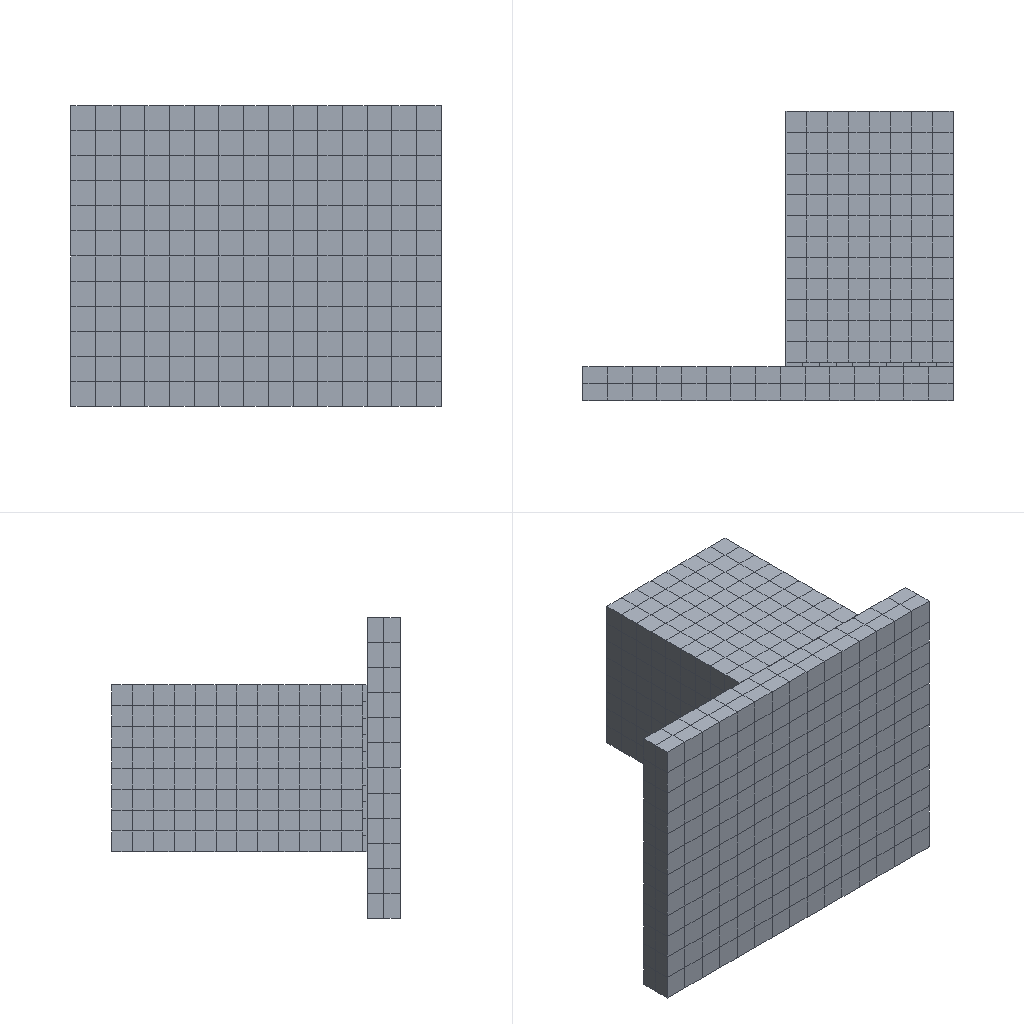Simulation study | ansys workbench
Ansys APDL input file, long lists of numbers shortened:
/batch
/config,noeldb,1     ! force off writing results to database
*get,_wallstrt,active,,time,wall
! ANSYS input file written by Workbench version 2022 R1
! File used for geometry attach:
/title,111--____ (F5)
! ****** Begin Custom Load Command Snippet ******
/COM, ACT Extensions:
/COM,     LSDYNA, 2021.1
/COM,
! ****** End   Custom Load Command Snippet ******
*DIM,_wb_ProjectScratch_dir,string,248
_wb_ProjectScratch_dir(1) = ''
*DIM,_wb_SolverFiles_dir,string,248
_wb_SolverFiles_dir(1) = ''
*DIM,_wb_userfiles_dir,string,248
_wb_userfiles_dir(1) = ''
/com,--- Data in consistent NMM units. See Solving Units in the help system for more information.
/units,MPA
/nopr
/wb,file,start              !  signify a WB generated input file
/prep7
! Turn off shape checking because checks already performed inside WB mesher.
! See help system for more information.
SHPP,OFF,,NOWARN
/nolist
etcon,set             ! allow ANSYS to choose best KEYOP's for 180x elements, resets any applicable keyopt to MAPDL defaults
/com,*********** Nodes for the whole assembly ***********
nblock,3,,7591
(1i9,3e20.9e3)
        1    -2.000000000E+00     0.000000000E+00    -2.000000000E+00
! (6900 more lines like these left out)
-1
/wb,elem,start            !  set before creation of elements
/com,*********** Elements for Body 1 "__2____1|NONE" ***********
et,1,186
keyo,1,2,1          ! set full integration on SOLID186
eblock,19,solid,,768
(19i9)
        1        1        1        1        0        0        0        0       20        0      461     3005     3858     3875     3882     3620     3859     3874     3959
! (1535 more lines like these left out)
-1
/com,*********** Elements for Body 2 "__5____1|NONE" ***********
et,2,186
keyo,2,2,1          ! set full integration on SOLID186
eblock,19,solid,,360
(19i9)
        2        2        2        2        0        0        0        0       20        0      101      804     1320     1348     1416     1111     1347     1349     1417
! (719 more lines like these left out)
-1
/com,*********** Elements for Body 3 "__3^___1|__-__1" ***********
et,3,186
keyo,3,2,1          ! set full integration on SOLID186
eblock,19,solid,,100
(19i9)
        3        3        3        3        0        0        0        0       20        0        1       81      222      223      224       82      183      182      181
! (199 more lines like these left out)
-1
/wb,elem,end               !  done creating elements
/com,*********** Send User Defined Coordinate System(s) ***********
csys,0
toffst,273.15,  ! Temperature offset from absolute zero
/com,*********** Set Reference Temperature ***********
tref,22.
/wb,mat,start              !  starting to send materials
/com,*********** Send Materials ***********
Temperature = 'TEMP' ! Temperature
MP,DENS,1,7.85e-09,	! tonne mm^-3
MP,ALPX,1,1.2e-05,	! C^-1
MP,C,1,434000000,	! mm^2 s^-2 C^-1
MP,KXX,1,60.5,	! tonne mm s^-3 C^-1
MP,RSVX,1,0.00017,	! ohm mm
MP,EX,1,200000,	! tonne s^-2 mm^-1
MP,NUXY,1,0.3,
MP,MURX,1,10000,
Temperature = 'TEMP' ! Temperature
MP,DENS,2,7.85e-09,	! tonne mm^-3
MP,ALPX,2,1.2e-05,	! C^-1
MP,C,2,434000000,	! mm^2 s^-2 C^-1
MP,KXX,2,60.5,	! tonne mm s^-3 C^-1
MP,RSVX,2,0.00017,	! ohm mm
MP,EX,2,200000,	! tonne s^-2 mm^-1
MP,NUXY,2,0.3,
MP,MURX,2,10000,
Temperature = 'TEMP' ! Temperature
MP,DENS,3,7.85e-09,	! tonne mm^-3
MP,ALPX,3,1.2e-05,	! C^-1
MP,C,3,434000000,	! mm^2 s^-2 C^-1
MP,KXX,3,60.5,	! tonne mm s^-3 C^-1
MP,RSVX,3,0.00017,	! ohm mm
MP,EX,3,200000,	! tonne s^-2 mm^-1
MP,NUXY,3,0.3,
MP,MURX,3,10000,
/wb,mat,end                !  done sending materials
!************************* Model Summary ********************
!__2____1|NONE,	结构钢,	matid,	1
!__5____1|NONE,	结构钢,	matid,	2
!__3^___1|__-__1,	结构钢,	matid,	3
!************************* End Model Summary ********************
! get the diagonal of the bounding box. Needed later for other things
*get,_xmin,node,,mnloc,x
*get,_ymin,node,,mnloc,y
*get,_zmin,node,,mnloc,z
*get,_xmax,node,,mxloc,x
*get,_ymax,node,,mxloc,y
*get,_zmax,node,,mxloc,z
_ASMDIAG=(_xmax-_xmin)*(_xmax-_xmin)+(_ymax-_ymin)*(_ymax-_ymin)+(_zmax-_zmin)*(_zmax-_zmin)
_ASMDIAG=SQRT(_ASMDIAG)
/wb,contact,start          !  starting to send contact
/com,*********** Create Contact "接触区域" ***********
/com,            Real Constant Set For Above Contact Is 5 & 4
*set,tid,5
*set,cid,4
r,tid
r,cid
et,tid,170
et,cid,174
eblock,10,,,64
(15i9)
     2449        5        5        5        0     3730     3738     3809     3729     6288     6304     6286     6285
! (63 more lines like these left out)
-1
eblock,10,,,64
(15i9)
     2513        4        4        4        0     3730     3738     3809     3729     6288     6304     6286     6285
! (63 more lines like these left out)
-1
eblock,10,,,100
(15i9)
     2577        4        5        4        0      222       81      224      223      502      503      785      784
! (99 more lines like these left out)
-1
eblock,10,,,100
(15i9)
     2677        5        4        5        0      222       81      224      223      502      503      785      784
! (99 more lines like these left out)
-1
keyo,cid,8,2               ! auto create asymmetric contact (from Program Controlled setting)
keyo,cid,10,0              ! adjust contact stiffness each NR iteration (from Program Controlled setting)
keyo,cid,12,5              ! bonded always
keyo,cid,2,0               ! augmented Lagrange
keyo,cid,4,0               ! on Gauss point (from Program Controlled setting)
keyo,cid,9,1               ! ignore initial gaps/penetration
keyo,cid,7,0               ! No Prediction
rmod,tid,3,10.      ! FKN
rmod,tid,5,0.       ! ICONT
rmod,tid,6,0.       ! PINB
rmod,tid,10,0.      ! CNOF
rmod,tid,12,0.      ! FKT
rmod,tid,36,33      ! WB DSID
rmod,cid,3,10.      ! FKN
rmod,cid,5,0.       ! ICONT
rmod,cid,6,0.       ! PINB
rmod,cid,10,0.      ! CNOF
rmod,cid,12,0.      ! FKT
rmod,cid,36,33      ! WB DSID
/com,*********** Create Contact "接触区域 2" ***********
/com,            Real Constant Set For Above Contact Is 7 & 6
*set,tid,7
*set,cid,6
r,tid
r,cid
et,tid,170
et,cid,174
eblock,10,,,56
(15i9)
     2777        7        7        7        0     1201     1202     1191     1190     2600     2580     2577     2578
! (55 more lines like these left out)
-1
eblock,10,,,56
(15i9)
     2833        6        6        6        0     1201     1202     1191     1190     2600     2580     2577     2578
! (55 more lines like these left out)
-1
eblock,10,,,100
(15i9)
     2889        6        7        6        0      181       82      183      182      506      507      723      721
! (99 more lines like these left out)
-1
eblock,10,,,100
(15i9)
     2989        7        6        7        0      181       82      183      182      506      507      723      721
! (99 more lines like these left out)
-1
keyo,cid,8,2               ! auto create asymmetric contact (from Program Controlled setting)
keyo,cid,10,0              ! adjust contact stiffness each NR iteration (from Program Controlled setting)
keyo,cid,12,5              ! bonded always
keyo,cid,2,0               ! augmented Lagrange
keyo,cid,4,0               ! on Gauss point (from Program Controlled setting)
keyo,cid,9,1               ! ignore initial gaps/penetration
keyo,cid,7,0               ! No Prediction
rmod,tid,3,10.      ! FKN
rmod,tid,5,0.       ! ICONT
rmod,tid,6,0.       ! PINB
rmod,tid,10,0.      ! CNOF
rmod,tid,12,0.      ! FKT
rmod,tid,36,36      ! WB DSID
rmod,cid,3,10.      ! FKN
rmod,cid,5,0.       ! ICONT
rmod,cid,6,0.       ! PINB
rmod,cid,10,0.      ! CNOF
rmod,cid,12,0.      ! FKT
rmod,cid,36,36      ! WB DSID
nsel,all
esel,all
/wb,contact,end            !  done creating contacts
/com,*********** Create Debonding "____" ***********
TB,CZM,4,1,,CBDE
TBDATA,1,1e-07,5e-06,8e-09,5e-06,0.1,0
TBDATA,7,2
*set,matid,4
/com,*********** Create Debonding "____ 2" ***********
TB,CZM,6,1,,CBDE
TBDATA,1,1e-07,5e-06,8e-09,5e-06,0.1,0
TBDATA,7,2
*set,matid,6
/golist
/wb,load,start             !  starting to send loads
/com,*********** Fixed Supports ***********
CMBLOCK,_FIXEDSU,NODE,      595
(8i10)
       958       959       960       961       962       963       964       965
! (74 more lines like these left out)
cmsel,s,_FIXEDSU
d,all,all
nsel,all
/com,*********** Define Force Using Surface Effect Elements ***********
local,12,0,0.,0.,0.,0.,0.,0.
csys,0
et,8,154
eblock,10,,,106
(15i9)
     3089        8        8        8       12     3721     3621     3719     3720     6053     6052     6266     6268
! (105 more lines like these left out)
-1
esel,s,type,,8
keyop,8,2,1                ! Apply load in local coordinate system
keyop,8,7,1                ! Use original area so load is constant in large deformation
esel,all
/gst,on,on
fini
*get,_numnode,node,0,count
*get,_numelem,elem,0,count
*get, _MAXELEMNUM, elem, 0, NUM, MAX
*get, _MAXNODENUM, node, 0, NUM, MAX
*get, _MAXELEMTYPE, etyp, 0, NUM, MAX
*get, _MAXREALCONST, real, 0, NUM, MAX
/go
/wb,load,end               !  done creating loads
/com,--- Number of total nodes = %_numnode%
/com,--- Number of contact elements = 746
/com,--- Number of spring elements = 0
/com,--- Number of bearing elements = 0
/com,--- Number of solid elements = 1228
/com,--- Number of condensed parts = 0
/com,--- Number of total elements = %_numelem%
*get,_wallbsol,active,,time,wall
/com,****************************************************************************
/com,*************************    SOLUTION       ********************************
/com,****************************************************************************
/solu
antype,0                   ! static analysis
_thickRatio=0.333   ! Ratio of thick parts in the model
eqsl,sparse,,,,,1
cntr,print,1               ! print out contact info and also make no initial contact an error
dmpoption,emat,no             ! Don't combine emat file for DANSYS
dmpoption,esav,no             ! Don't combine esav file for DANSYS
nldiag,cont,iter           ! print out contact info each equilibrium iteration
rescontrol,define,last,last,,dele	   ! Program Controlled
/com,****************************************************
/com,******************* SOLVE FOR LS 1 OF 1 ****************
esel,s,type,,8
nsle
sfe,all,1,pres,1,13.089
sfe,all,2,pres,1,0.
sfe,all,3,pres,1,-2.2705804659384e-015
nsel,all
esel,all
/nopr
/gopr
autots,on                  ! Workbench Program Controlled automatic time stepping
nsub,5,1000,1              ! due to presence of nonlinear materials
time,1.
outres,erase
outres,all,none
outres,nsol,all,
outres,rsol,all
outres,eangl,all
outres,etmp,all
outres,veng,all
outres,strs,all,
outres,epel,all,
outres,eppl,all,
outres,cont,all,
! *********** WB SOLVE COMMAND ***********
! check interactive state
*get,ANSINTER_,active,,int
*if,ANSINTER_,ne,0,then
/eof
*endif
solve
/com *************** Write FE CONNECTORS *********
CEWRITE,file,ce,,INTE
/com,****************************************************
/com,*************** FINISHED SOLVE FOR LS 1 *************
*get,_wallasol,active,,time,wall
/nopr
*get,_numnode,node,0,count
*get,_numelem,elem,0,count
*get, _MAXELEMNUM, elem, 0, NUM, MAX
*get, _MAXNODENUM, node, 0, NUM, MAX,,,INTERNAL
*get, _MAXELEMTYPE, etyp, 0, NUM, MAX
*get, _MAXREALCONST, real, 0, NUM, MAX
/gopr
/post1
xmlo,ENCODING,ISO-8859-1
xmlo,parm
/xml,parm,xml
fini
/gopr
*get,_walldone,active,,time,wall
_preptime=(_wallbsol-_wallstrt)*3600
_solvtime=(_wallasol-_wallbsol)*3600
_posttime=(_walldone-_wallasol)*3600
_totaltim=(_walldone-_wallstrt)*3600
*get,_dlbratio,active,0,solu,dlbr
*get,_combtime,active,0,solu,comb
*get,_ssmode,active,0,solu,ssmm
*get,_ndofs,active,0,solu,ndof
*get,_sol_end_time,active,0,set,time
*if,_sol_end_time,eq,1.,then
/fclean				!clean distributed files
*endif
/com,--- Total number of nodes = %_numnode%
/com,--- Total number of elements = %_numelem%
/com,--- Element load balance ratio = %_dlbratio%
/com,--- Time to combine distributed files = %_combtime%
/com,--- Sparse memory mode = %_ssmode%
/com,--- Number of DOF = %_ndofs%
/wb,file,end               ! done with WB generated input